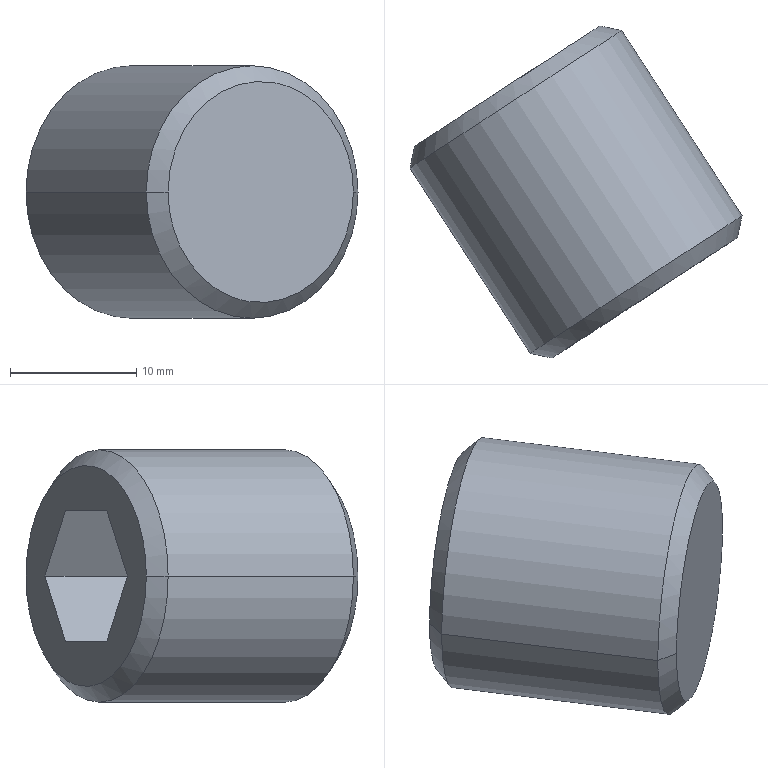Part | STEP file | Buj_o_1-A | 1 solid | 15 faces | box 26.305 x 26.305 x 20 mm | volume 4786 mm3 | plane 9 | cone 4 | cylinder 2 | commonest cylinder face diameters 20 x2
STEP:
#1=CARTESIAN_POINT('',(0.,0.,0.));
#2=DIRECTION('',(0.,0.,1.));
#3=DIRECTION('',(1.,0.,0.));
#4=AXIS2_PLACEMENT_3D('',#1,#2,#3);
#5=CARTESIAN_POINT('',(-85.7,150.327,23.));
#6=VERTEX_POINT('',#5);
#7=CARTESIAN_POINT('',(-102.473,139.434,23.));
#8=VERTEX_POINT('',#7);
#9=CARTESIAN_POINT('',(-94.086,144.88,23.));
#10=DIRECTION('',(0.5446,-0.8387,0.));
#11=DIRECTION('',(0.8387,0.5446,0.));
#12=AXIS2_PLACEMENT_3D('',#9,#10,#11);
#13=CIRCLE('',#12,10.);
#14=CARTESIAN_POINT('',(-94.767,145.929,23.));
#15=DIRECTION('',(0.5446,-0.8387,0.));
#16=DIRECTION('',(0.8387,0.5446,0.));
#17=AXIS2_PLACEMENT_3D('',#14,#15,#16);
#18=CYLINDRICAL_SURFACE('',#17,10.);
#19=CARTESIAN_POINT('',(0.,1.25));
#20=DIRECTION('',(1.,0.));
#21=VECTOR('',#20,1.);
#22=LINE('',#19,#21);
#23=(GEOMETRIC_REPRESENTATION_CONTEXT(2)PARAMETRIC_REPRESENTATION_CONTEXT()REPRESENTATION_CONTEXT('',''));
#24=DEFINITIONAL_REPRESENTATION('',(#22),#23);
#25=PCURVE('',#18,#24);
#26=CARTESIAN_POINT('',(-94.086,144.88,23.));
#27=DIRECTION('',(0.5446,-0.8387,0.));
#28=DIRECTION('',(0.8387,0.5446,0.));
#29=AXIS2_PLACEMENT_3D('',#26,#27,#28);
#30=CONICAL_SURFACE('',#29,10.,0.7854);
#31=CARTESIAN_POINT('',(0.,0.));
#32=DIRECTION('',(1.,0.));
#33=VECTOR('',#32,1.);
#34=LINE('',#31,#33);
#35=(GEOMETRIC_REPRESENTATION_CONTEXT(2)PARAMETRIC_REPRESENTATION_CONTEXT()REPRESENTATION_CONTEXT('',''));
#36=DEFINITIONAL_REPRESENTATION('',(#34),#35);
#37=PCURVE('',#30,#36);
#38=SURFACE_CURVE('',#13,(#25,#37),.PCURVE_S1.);
#39=EDGE_CURVE('',#6,#8,#38,.T.);
#40=ORIENTED_EDGE('',*,*,#39,.T.);
#41=CARTESIAN_POINT('',(-92.942,124.757,23.));
#42=VERTEX_POINT('',#41);
#43=CARTESIAN_POINT('',(-103.154,140.482,23.));
#44=DIRECTION('',(0.5446,-0.8387,0.));
#45=VECTOR('',#44,1.);
#46=LINE('',#43,#45);
#47=CARTESIAN_POINT('',(3.142,0.));
#48=DIRECTION('',(0.,1.));
#49=VECTOR('',#48,1.);
#50=LINE('',#47,#49);
#51=(GEOMETRIC_REPRESENTATION_CONTEXT(2)PARAMETRIC_REPRESENTATION_CONTEXT()REPRESENTATION_CONTEXT('',''));
#52=DEFINITIONAL_REPRESENTATION('',(#50),#51);
#53=PCURVE('',#18,#52);
#54=CARTESIAN_POINT('',(-94.767,145.929,23.));
#55=DIRECTION('',(0.5446,-0.8387,0.));
#56=DIRECTION('',(0.8387,0.5446,0.));
#57=AXIS2_PLACEMENT_3D('',#54,#55,#56);
#58=CYLINDRICAL_SURFACE('',#57,10.);
#59=CARTESIAN_POINT('',(3.142,0.));
#60=DIRECTION('',(0.,1.));
#61=VECTOR('',#60,1.);
#62=LINE('',#59,#61);
#63=(GEOMETRIC_REPRESENTATION_CONTEXT(2)PARAMETRIC_REPRESENTATION_CONTEXT()REPRESENTATION_CONTEXT('',''));
#64=DEFINITIONAL_REPRESENTATION('',(#62),#63);
#65=PCURVE('',#58,#64);
#66=SURFACE_CURVE('',#46,(#53,#65),.PCURVE_S1.);
#67=EDGE_CURVE('',#8,#42,#66,.T.);
#68=ORIENTED_EDGE('',*,*,#67,.T.);
#69=CARTESIAN_POINT('',(-76.169,135.65,23.));
#70=VERTEX_POINT('',#69);
#71=CARTESIAN_POINT('',(-84.555,130.204,23.));
#72=DIRECTION('',(-0.5446,0.8387,0.));
#73=DIRECTION('',(0.8387,0.5446,0.));
#74=AXIS2_PLACEMENT_3D('',#71,#72,#73);
#75=CIRCLE('',#74,10.);
#76=CARTESIAN_POINT('',(6.283,18.75));
#77=DIRECTION('',(-1.,0.));
#78=VECTOR('',#77,1.);
#79=LINE('',#76,#78);
#80=(GEOMETRIC_REPRESENTATION_CONTEXT(2)PARAMETRIC_REPRESENTATION_CONTEXT()REPRESENTATION_CONTEXT('',''));
#81=DEFINITIONAL_REPRESENTATION('',(#79),#80);
#82=PCURVE('',#18,#81);
#83=CARTESIAN_POINT('',(-84.555,130.204,23.));
#84=DIRECTION('',(-0.5446,0.8387,0.));
#85=DIRECTION('',(-0.8387,-0.5446,0.));
#86=AXIS2_PLACEMENT_3D('',#83,#84,#85);
#87=CONICAL_SURFACE('',#86,10.,0.7854);
#88=CARTESIAN_POINT('',(-3.142,0.));
#89=DIRECTION('',(1.,0.));
#90=VECTOR('',#89,1.);
#91=LINE('',#88,#90);
#92=(GEOMETRIC_REPRESENTATION_CONTEXT(2)PARAMETRIC_REPRESENTATION_CONTEXT()REPRESENTATION_CONTEXT('',''));
#93=DEFINITIONAL_REPRESENTATION('',(#91),#92);
#94=PCURVE('',#87,#93);
#95=SURFACE_CURVE('',#75,(#82,#94),.PCURVE_S1.);
#96=EDGE_CURVE('',#42,#70,#95,.T.);
#97=ORIENTED_EDGE('',*,*,#96,.T.);
#98=CARTESIAN_POINT('',(-86.38,151.375,23.));
#99=DIRECTION('',(0.5446,-0.8387,0.));
#100=VECTOR('',#99,1.);
#101=LINE('',#98,#100);
#102=CARTESIAN_POINT('',(0.,0.));
#103=DIRECTION('',(0.,1.));
#104=VECTOR('',#103,1.);
#105=LINE('',#102,#104);
#106=(GEOMETRIC_REPRESENTATION_CONTEXT(2)PARAMETRIC_REPRESENTATION_CONTEXT()REPRESENTATION_CONTEXT('',''));
#107=DEFINITIONAL_REPRESENTATION('',(#105),#106);
#108=PCURVE('',#18,#107);
#109=CARTESIAN_POINT('',(6.283,0.));
#110=DIRECTION('',(0.,1.));
#111=VECTOR('',#110,1.);
#112=LINE('',#109,#111);
#113=(GEOMETRIC_REPRESENTATION_CONTEXT(2)PARAMETRIC_REPRESENTATION_CONTEXT()REPRESENTATION_CONTEXT('',''));
#114=DEFINITIONAL_REPRESENTATION('',(#112),#113);
#115=PCURVE('',#58,#114);
#116=SURFACE_CURVE('',#101,(#108,#115),.PCURVE_S1.);
#117=EDGE_CURVE('',#6,#70,#116,.T.);
#118=ORIENTED_EDGE('',*,*,#117,.F.);
#119=EDGE_LOOP('',(#40,#68,#97,#118));
#120=FACE_BOUND('',#119,.T.);
#121=ADVANCED_FACE('',(#120),#18,.T.);
#122=CARTESIAN_POINT('',(-91.213,124.39,23.));
#123=VERTEX_POINT('',#122);
#124=CARTESIAN_POINT('',(-76.536,133.921,23.));
#125=VERTEX_POINT('',#124);
#126=CARTESIAN_POINT('',(-91.213,124.39,23.));
#127=CARTESIAN_POINT('',(-91.213,124.39,24.145));
#128=CARTESIAN_POINT('',(-91.022,124.514,25.29));
#129=CARTESIAN_POINT('',(-90.287,124.991,27.407));
#130=CARTESIAN_POINT('',(-89.743,125.344,28.377));
#131=CARTESIAN_POINT('',(-88.384,126.227,29.997));
#132=CARTESIAN_POINT('',(-87.57,126.755,30.646));
#133=CARTESIAN_POINT('',(-85.795,127.908,31.522));
#134=CARTESIAN_POINT('',(-84.835,128.531,31.75));
#135=CARTESIAN_POINT('',(-82.914,129.779,31.75));
#136=CARTESIAN_POINT('',(-81.954,130.403,31.522));
#137=CARTESIAN_POINT('',(-80.179,131.555,30.646));
#138=CARTESIAN_POINT('',(-79.365,132.084,29.997));
#139=CARTESIAN_POINT('',(-78.006,132.966,28.377));
#140=CARTESIAN_POINT('',(-77.462,133.319,27.407));
#141=CARTESIAN_POINT('',(-76.727,133.797,25.29));
#142=CARTESIAN_POINT('',(-76.536,133.921,24.145));
#143=CARTESIAN_POINT('',(-76.536,133.921,23.));
#144=B_SPLINE_CURVE_WITH_KNOTS('',3,(#126,#127,#128,#129,#130,#131,#132,#133,#134,#135,#136,#137,#138,#139,#140,#141,#142,#143),.UNSPECIFIED.,.F.,.F.,(4,2,2,2,2,2,2,2,4),(0.75,0.8125,0.875,0.9375,1.,1.062,1.125,1.188,1.25),.UNSPECIFIED.);
#145=CARTESIAN_POINT('',(0.,-1.25));
#146=CARTESIAN_POINT('',(0.0238,-1.25));
#147=CARTESIAN_POINT('',(0.0714,-1.25));
#148=CARTESIAN_POINT('',(0.1428,-1.25));
#149=CARTESIAN_POINT('',(0.2142,-1.25));
#150=CARTESIAN_POINT('',(0.2856,-1.25));
#151=CARTESIAN_POINT('',(0.357,-1.25));
#152=CARTESIAN_POINT('',(0.4284,-1.25));
#153=CARTESIAN_POINT('',(0.4998,-1.25));
#154=CARTESIAN_POINT('',(0.5712,-1.25));
#155=CARTESIAN_POINT('',(0.6426,-1.25));
#156=CARTESIAN_POINT('',(0.714,-1.25));
#157=CARTESIAN_POINT('',(0.7854,-1.25));
#158=CARTESIAN_POINT('',(0.8568,-1.25));
#159=CARTESIAN_POINT('',(0.9282,-1.25));
#160=CARTESIAN_POINT('',(0.9996,-1.25));
#161=CARTESIAN_POINT('',(1.071,-1.25));
#162=CARTESIAN_POINT('',(1.142,-1.25));
#163=CARTESIAN_POINT('',(1.214,-1.25));
#164=CARTESIAN_POINT('',(1.285,-1.25));
#165=CARTESIAN_POINT('',(1.357,-1.25));
#166=CARTESIAN_POINT('',(1.428,-1.25));
#167=CARTESIAN_POINT('',(1.499,-1.25));
#168=CARTESIAN_POINT('',(1.571,-1.25));
#169=CARTESIAN_POINT('',(1.642,-1.25));
#170=CARTESIAN_POINT('',(1.714,-1.25));
#171=CARTESIAN_POINT('',(1.785,-1.25));
#172=CARTESIAN_POINT('',(1.856,-1.25));
#173=CARTESIAN_POINT('',(1.928,-1.25));
#174=CARTESIAN_POINT('',(1.999,-1.25));
#175=CARTESIAN_POINT('',(2.071,-1.25));
#176=CARTESIAN_POINT('',(2.142,-1.25));
#177=CARTESIAN_POINT('',(2.213,-1.25));
#178=CARTESIAN_POINT('',(2.285,-1.25));
#179=CARTESIAN_POINT('',(2.356,-1.25));
#180=CARTESIAN_POINT('',(2.428,-1.25));
#181=CARTESIAN_POINT('',(2.499,-1.25));
#182=CARTESIAN_POINT('',(2.57,-1.25));
#183=CARTESIAN_POINT('',(2.642,-1.25));
#184=CARTESIAN_POINT('',(2.713,-1.25));
#185=CARTESIAN_POINT('',(2.785,-1.25));
#186=CARTESIAN_POINT('',(2.856,-1.25));
#187=CARTESIAN_POINT('',(2.927,-1.25));
#188=CARTESIAN_POINT('',(2.999,-1.25));
#189=CARTESIAN_POINT('',(3.07,-1.25));
#190=CARTESIAN_POINT('',(3.118,-1.25));
#191=CARTESIAN_POINT('',(3.142,-1.25));
#192=B_SPLINE_CURVE_WITH_KNOTS('',3,(#145,#146,#147,#148,#149,#150,#151,#152,#153,#154,#155,#156,#157,#158,#159,#160,#161,#162,#163,#164,#165,#166,#167,#168,#169,#170,#171,#172,#173,#174,#175,#176,#177,#178,#179,#180,#181,#182,#183,#184,#185,#186,#187,#188,#189,#190,#191),.UNSPECIFIED.,.F.,.F.,(4,1,1,1,1,1,1,1,1,1,1,1,1,1,1,1,1,1,1,1,1,1,1,1,1,1,1,1,1,1,1,1,1,1,1,1,1,1,1,1,1,1,1,1,4),(0.75,0.7614,0.7727,0.7841,0.7955,0.8068,0.8182,0.8295,0.8409,0.8523,0.8636,0.875,0.8864,0.8977,0.9091,0.9205,0.9318,0.9432,0.9545,0.9659,0.9773,0.9886,1.,1.011,1.023,1.034,1.045,1.057,1.068,1.08,1.091,1.102,1.114,1.125,1.136,1.148,1.159,1.17,1.182,1.193,1.205,1.216,1.227,1.239,1.25),.QUASI_UNIFORM_KNOTS.);
#193=(GEOMETRIC_REPRESENTATION_CONTEXT(2)PARAMETRIC_REPRESENTATION_CONTEXT()REPRESENTATION_CONTEXT('',''));
#194=DEFINITIONAL_REPRESENTATION('',(#192),#193);
#195=PCURVE('',#87,#194);
#196=CARTESIAN_POINT('',(-83.874,129.155,23.));
#197=DIRECTION('',(0.5446,-0.8387,0.));
#198=DIRECTION('',(0.8387,0.5446,0.));
#199=AXIS2_PLACEMENT_3D('',#196,#197,#198);
#200=PLANE('',#199);
#201=CARTESIAN_POINT('',(-8.75,0.));
#202=CARTESIAN_POINT('',(-8.75,1.145));
#203=CARTESIAN_POINT('',(-8.522,2.29));
#204=CARTESIAN_POINT('',(-7.646,4.407));
#205=CARTESIAN_POINT('',(-6.997,5.377));
#206=CARTESIAN_POINT('',(-5.377,6.997));
#207=CARTESIAN_POINT('',(-4.407,7.646));
#208=CARTESIAN_POINT('',(-2.29,8.522));
#209=CARTESIAN_POINT('',(-1.145,8.75));
#210=CARTESIAN_POINT('',(1.145,8.75));
#211=CARTESIAN_POINT('',(2.29,8.522));
#212=CARTESIAN_POINT('',(4.407,7.646));
#213=CARTESIAN_POINT('',(5.377,6.997));
#214=CARTESIAN_POINT('',(6.997,5.377));
#215=CARTESIAN_POINT('',(7.646,4.407));
#216=CARTESIAN_POINT('',(8.522,2.29));
#217=CARTESIAN_POINT('',(8.75,1.145));
#218=CARTESIAN_POINT('',(8.75,0.));
#219=B_SPLINE_CURVE_WITH_KNOTS('',3,(#201,#202,#203,#204,#205,#206,#207,#208,#209,#210,#211,#212,#213,#214,#215,#216,#217,#218),.UNSPECIFIED.,.F.,.F.,(4,2,2,2,2,2,2,2,4),(0.75,0.8125,0.875,0.9375,1.,1.062,1.125,1.188,1.25),.UNSPECIFIED.);
#220=(GEOMETRIC_REPRESENTATION_CONTEXT(2)PARAMETRIC_REPRESENTATION_CONTEXT()REPRESENTATION_CONTEXT('',''));
#221=DEFINITIONAL_REPRESENTATION('',(#219),#220);
#222=PCURVE('',#200,#221);
#223=SURFACE_CURVE('',#144,(#195,#222),.PCURVE_S1.);
#224=EDGE_CURVE('',#123,#125,#223,.T.);
#225=ORIENTED_EDGE('',*,*,#224,.T.);
#226=CARTESIAN_POINT('',(-76.169,135.65,23.));
#227=DIRECTION('',(0.2079,0.9781,0.));
#228=VECTOR('',#227,1.);
#229=LINE('',#226,#228);
#230=CARTESIAN_POINT('',(3.142,0.));
#231=DIRECTION('',(0.,1.));
#232=VECTOR('',#231,1.);
#233=LINE('',#230,#232);
#234=(GEOMETRIC_REPRESENTATION_CONTEXT(2)PARAMETRIC_REPRESENTATION_CONTEXT()REPRESENTATION_CONTEXT('',''));
#235=DEFINITIONAL_REPRESENTATION('',(#233),#234);
#236=PCURVE('',#87,#235);
#237=CARTESIAN_POINT('',(-84.555,130.204,23.));
#238=DIRECTION('',(-0.5446,0.8387,0.));
#239=DIRECTION('',(-0.8387,-0.5446,0.));
#240=AXIS2_PLACEMENT_3D('',#237,#238,#239);
#241=CONICAL_SURFACE('',#240,10.,0.7854);
#242=CARTESIAN_POINT('',(3.142,0.));
#243=DIRECTION('',(0.,1.));
#244=VECTOR('',#243,1.);
#245=LINE('',#242,#244);
#246=(GEOMETRIC_REPRESENTATION_CONTEXT(2)PARAMETRIC_REPRESENTATION_CONTEXT()REPRESENTATION_CONTEXT('',''));
#247=DEFINITIONAL_REPRESENTATION('',(#245),#246);
#248=PCURVE('',#241,#247);
#249=SURFACE_CURVE('',#229,(#236,#248),.PCURVE_S1.);
#250=EDGE_CURVE('',#125,#70,#249,.T.);
#251=ORIENTED_EDGE('',*,*,#250,.T.);
#252=ORIENTED_EDGE('',*,*,#96,.F.);
#253=CARTESIAN_POINT('',(-92.942,124.757,23.));
#254=DIRECTION('',(-0.9781,0.2079,0.));
#255=VECTOR('',#254,1.);
#256=LINE('',#253,#255);
#257=CARTESIAN_POINT('',(0.,0.));
#258=DIRECTION('',(0.,1.));
#259=VECTOR('',#258,1.);
#260=LINE('',#257,#259);
#261=(GEOMETRIC_REPRESENTATION_CONTEXT(2)PARAMETRIC_REPRESENTATION_CONTEXT()REPRESENTATION_CONTEXT('',''));
#262=DEFINITIONAL_REPRESENTATION('',(#260),#261);
#263=PCURVE('',#87,#262);
#264=CARTESIAN_POINT('',(6.283,0.));
#265=DIRECTION('',(0.,1.));
#266=VECTOR('',#265,1.);
#267=LINE('',#264,#266);
#268=(GEOMETRIC_REPRESENTATION_CONTEXT(2)PARAMETRIC_REPRESENTATION_CONTEXT()REPRESENTATION_CONTEXT('',''));
#269=DEFINITIONAL_REPRESENTATION('',(#267),#268);
#270=PCURVE('',#241,#269);
#271=SURFACE_CURVE('',#256,(#263,#270),.PCURVE_S1.);
#272=EDGE_CURVE('',#123,#42,#271,.T.);
#273=ORIENTED_EDGE('',*,*,#272,.F.);
#274=EDGE_LOOP('',(#225,#251,#252,#273));
#275=FACE_BOUND('',#274,.T.);
#276=ADVANCED_FACE('',(#275),#87,.T.);
#277=CARTESIAN_POINT('',(-87.429,150.694,23.));
#278=VERTEX_POINT('',#277);
#279=CARTESIAN_POINT('',(-102.106,141.163,23.));
#280=VERTEX_POINT('',#279);
#281=CARTESIAN_POINT('',(-87.429,150.694,23.));
#282=CARTESIAN_POINT('',(-87.429,150.694,24.145));
#283=CARTESIAN_POINT('',(-87.62,150.57,25.29));
#284=CARTESIAN_POINT('',(-88.355,150.093,27.407));
#285=CARTESIAN_POINT('',(-88.899,149.74,28.377));
#286=CARTESIAN_POINT('',(-90.257,148.857,29.997));
#287=CARTESIAN_POINT('',(-91.071,148.329,30.646));
#288=CARTESIAN_POINT('',(-92.846,147.176,31.522));
#289=CARTESIAN_POINT('',(-93.807,146.552,31.75));
#290=CARTESIAN_POINT('',(-95.728,145.305,31.75));
#291=CARTESIAN_POINT('',(-96.688,144.681,31.522));
#292=CARTESIAN_POINT('',(-98.463,143.529,30.646));
#293=CARTESIAN_POINT('',(-99.277,143.,29.997));
#294=CARTESIAN_POINT('',(-100.635,142.118,28.377));
#295=CARTESIAN_POINT('',(-101.179,141.765,27.407));
#296=CARTESIAN_POINT('',(-101.915,141.287,25.29));
#297=CARTESIAN_POINT('',(-102.106,141.163,24.145));
#298=CARTESIAN_POINT('',(-102.106,141.163,23.));
#299=B_SPLINE_CURVE_WITH_KNOTS('',3,(#281,#282,#283,#284,#285,#286,#287,#288,#289,#290,#291,#292,#293,#294,#295,#296,#297,#298),.UNSPECIFIED.,.F.,.F.,(4,2,2,2,2,2,2,2,4),(0.25,0.3125,0.375,0.4375,0.5,0.5625,0.625,0.6875,0.75),.UNSPECIFIED.);
#300=CARTESIAN_POINT('',(0.,-1.25));
#301=CARTESIAN_POINT('',(0.0238,-1.25));
#302=CARTESIAN_POINT('',(0.0714,-1.25));
#303=CARTESIAN_POINT('',(0.1428,-1.25));
#304=CARTESIAN_POINT('',(0.2142,-1.25));
#305=CARTESIAN_POINT('',(0.2856,-1.25));
#306=CARTESIAN_POINT('',(0.357,-1.25));
#307=CARTESIAN_POINT('',(0.4284,-1.25));
#308=CARTESIAN_POINT('',(0.4998,-1.25));
#309=CARTESIAN_POINT('',(0.5712,-1.25));
#310=CARTESIAN_POINT('',(0.6426,-1.25));
#311=CARTESIAN_POINT('',(0.714,-1.25));
#312=CARTESIAN_POINT('',(0.7854,-1.25));
#313=CARTESIAN_POINT('',(0.8568,-1.25));
#314=CARTESIAN_POINT('',(0.9282,-1.25));
#315=CARTESIAN_POINT('',(0.9996,-1.25));
#316=CARTESIAN_POINT('',(1.071,-1.25));
#317=CARTESIAN_POINT('',(1.142,-1.25));
#318=CARTESIAN_POINT('',(1.214,-1.25));
#319=CARTESIAN_POINT('',(1.285,-1.25));
#320=CARTESIAN_POINT('',(1.357,-1.25));
#321=CARTESIAN_POINT('',(1.428,-1.25));
#322=CARTESIAN_POINT('',(1.499,-1.25));
#323=CARTESIAN_POINT('',(1.571,-1.25));
#324=CARTESIAN_POINT('',(1.642,-1.25));
#325=CARTESIAN_POINT('',(1.714,-1.25));
#326=CARTESIAN_POINT('',(1.785,-1.25));
#327=CARTESIAN_POINT('',(1.856,-1.25));
#328=CARTESIAN_POINT('',(1.928,-1.25));
#329=CARTESIAN_POINT('',(1.999,-1.25));
#330=CARTESIAN_POINT('',(2.071,-1.25));
#331=CARTESIAN_POINT('',(2.142,-1.25));
#332=CARTESIAN_POINT('',(2.213,-1.25));
#333=CARTESIAN_POINT('',(2.285,-1.25));
#334=CARTESIAN_POINT('',(2.356,-1.25));
#335=CARTESIAN_POINT('',(2.428,-1.25));
#336=CARTESIAN_POINT('',(2.499,-1.25));
#337=CARTESIAN_POINT('',(2.57,-1.25));
#338=CARTESIAN_POINT('',(2.642,-1.25));
#339=CARTESIAN_POINT('',(2.713,-1.25));
#340=CARTESIAN_POINT('',(2.785,-1.25));
#341=CARTESIAN_POINT('',(2.856,-1.25));
#342=CARTESIAN_POINT('',(2.927,-1.25));
#343=CARTESIAN_POINT('',(2.999,-1.25));
#344=CARTESIAN_POINT('',(3.07,-1.25));
#345=CARTESIAN_POINT('',(3.118,-1.25));
#346=CARTESIAN_POINT('',(3.142,-1.25));
#347=B_SPLINE_CURVE_WITH_KNOTS('',3,(#300,#301,#302,#303,#304,#305,#306,#307,#308,#309,#310,#311,#312,#313,#314,#315,#316,#317,#318,#319,#320,#321,#322,#323,#324,#325,#326,#327,#328,#329,#330,#331,#332,#333,#334,#335,#336,#337,#338,#339,#340,#341,#342,#343,#344,#345,#346),.UNSPECIFIED.,.F.,.F.,(4,1,1,1,1,1,1,1,1,1,1,1,1,1,1,1,1,1,1,1,1,1,1,1,1,1,1,1,1,1,1,1,1,1,1,1,1,1,1,1,1,1,1,1,4),(0.25,0.2614,0.2727,0.2841,0.2955,0.3068,0.3182,0.3295,0.3409,0.3523,0.3636,0.375,0.3864,0.3977,0.4091,0.4205,0.4318,0.4432,0.4545,0.4659,0.4773,0.4886,0.5,0.5114,0.5227,0.5341,0.5455,0.5568,0.5682,0.5795,0.5909,0.6023,0.6136,0.625,0.6364,0.6477,0.6591,0.6705,0.6818,0.6932,0.7045,0.7159,0.7273,0.7386,0.75),.QUASI_UNIFORM_KNOTS.);
#348=(GEOMETRIC_REPRESENTATION_CONTEXT(2)PARAMETRIC_REPRESENTATION_CONTEXT()REPRESENTATION_CONTEXT('',''));
#349=DEFINITIONAL_REPRESENTATION('',(#347),#348);
#350=PCURVE('',#30,#349);
#351=CARTESIAN_POINT('',(-94.767,145.929,23.));
#352=DIRECTION('',(-0.5446,0.8387,0.));
#353=DIRECTION('',(-0.8387,-0.5446,0.));
#354=AXIS2_PLACEMENT_3D('',#351,#352,#353);
#355=PLANE('',#354);
#356=CARTESIAN_POINT('',(-8.75,0.));
#357=CARTESIAN_POINT('',(-8.75,1.145));
#358=CARTESIAN_POINT('',(-8.522,2.29));
#359=CARTESIAN_POINT('',(-7.646,4.407));
#360=CARTESIAN_POINT('',(-6.997,5.377));
#361=CARTESIAN_POINT('',(-5.377,6.997));
#362=CARTESIAN_POINT('',(-4.407,7.646));
#363=CARTESIAN_POINT('',(-2.29,8.522));
#364=CARTESIAN_POINT('',(-1.145,8.75));
#365=CARTESIAN_POINT('',(1.145,8.75));
#366=CARTESIAN_POINT('',(2.29,8.522));
#367=CARTESIAN_POINT('',(4.407,7.646));
#368=CARTESIAN_POINT('',(5.377,6.997));
#369=CARTESIAN_POINT('',(6.997,5.377));
#370=CARTESIAN_POINT('',(7.646,4.407));
#371=CARTESIAN_POINT('',(8.522,2.29));
#372=CARTESIAN_POINT('',(8.75,1.145));
#373=CARTESIAN_POINT('',(8.75,0.));
#374=B_SPLINE_CURVE_WITH_KNOTS('',3,(#356,#357,#358,#359,#360,#361,#362,#363,#364,#365,#366,#367,#368,#369,#370,#371,#372,#373),.UNSPECIFIED.,.F.,.F.,(4,2,2,2,2,2,2,2,4),(0.25,0.3125,0.375,0.4375,0.5,0.5625,0.625,0.6875,0.75),.UNSPECIFIED.);
#375=(GEOMETRIC_REPRESENTATION_CONTEXT(2)PARAMETRIC_REPRESENTATION_CONTEXT()REPRESENTATION_CONTEXT('',''));
#376=DEFINITIONAL_REPRESENTATION('',(#374),#375);
#377=PCURVE('',#355,#376);
#378=SURFACE_CURVE('',#299,(#350,#377),.PCURVE_S1.);
#379=EDGE_CURVE('',#278,#280,#378,.T.);
#380=ORIENTED_EDGE('',*,*,#379,.T.);
#381=CARTESIAN_POINT('',(-102.473,139.434,23.));
#382=DIRECTION('',(-0.2079,-0.9781,0.));
#383=VECTOR('',#382,1.);
#384=LINE('',#381,#383);
#385=CARTESIAN_POINT('',(3.142,0.));
#386=DIRECTION('',(0.,1.));
#387=VECTOR('',#386,1.);
#388=LINE('',#385,#387);
#389=(GEOMETRIC_REPRESENTATION_CONTEXT(2)PARAMETRIC_REPRESENTATION_CONTEXT()REPRESENTATION_CONTEXT('',''));
#390=DEFINITIONAL_REPRESENTATION('',(#388),#389);
#391=PCURVE('',#30,#390);
#392=CARTESIAN_POINT('',(-94.086,144.88,23.));
#393=DIRECTION('',(0.5446,-0.8387,0.));
#394=DIRECTION('',(0.8387,0.5446,0.));
#395=AXIS2_PLACEMENT_3D('',#392,#393,#394);
#396=CONICAL_SURFACE('',#395,10.,0.7854);
#397=CARTESIAN_POINT('',(3.142,0.));
#398=DIRECTION('',(0.,1.));
#399=VECTOR('',#398,1.);
#400=LINE('',#397,#399);
#401=(GEOMETRIC_REPRESENTATION_CONTEXT(2)PARAMETRIC_REPRESENTATION_CONTEXT()REPRESENTATION_CONTEXT('',''));
#402=DEFINITIONAL_REPRESENTATION('',(#400),#401);
#403=PCURVE('',#396,#402);
#404=SURFACE_CURVE('',#384,(#391,#403),.PCURVE_S1.);
#405=EDGE_CURVE('',#280,#8,#404,.T.);
#406=ORIENTED_EDGE('',*,*,#405,.T.);
#407=ORIENTED_EDGE('',*,*,#39,.F.);
#408=CARTESIAN_POINT('',(-85.7,150.327,23.));
#409=DIRECTION('',(0.9781,-0.2079,0.));
#410=VECTOR('',#409,1.);
#411=LINE('',#408,#410);
#412=CARTESIAN_POINT('',(0.,0.));
#413=DIRECTION('',(0.,1.));
#414=VECTOR('',#413,1.);
#415=LINE('',#412,#414);
#416=(GEOMETRIC_REPRESENTATION_CONTEXT(2)PARAMETRIC_REPRESENTATION_CONTEXT()REPRESENTATION_CONTEXT('',''));
#417=DEFINITIONAL_REPRESENTATION('',(#415),#416);
#418=PCURVE('',#30,#417);
#419=CARTESIAN_POINT('',(6.283,0.));
#420=DIRECTION('',(0.,1.));
#421=VECTOR('',#420,1.);
#422=LINE('',#419,#421);
#423=(GEOMETRIC_REPRESENTATION_CONTEXT(2)PARAMETRIC_REPRESENTATION_CONTEXT()REPRESENTATION_CONTEXT('',''));
#424=DEFINITIONAL_REPRESENTATION('',(#422),#423);
#425=PCURVE('',#396,#424);
#426=SURFACE_CURVE('',#411,(#418,#425),.PCURVE_S1.);
#427=EDGE_CURVE('',#278,#6,#426,.T.);
#428=ORIENTED_EDGE('',*,*,#427,.F.);
#429=EDGE_LOOP('',(#380,#406,#407,#428));
#430=FACE_BOUND('',#429,.T.);
#431=ADVANCED_FACE('',(#430),#30,.T.);
#432=ORIENTED_EDGE('',*,*,#67,.F.);
#433=CARTESIAN_POINT('',(-94.086,144.88,23.));
#434=DIRECTION('',(0.5446,-0.8387,0.));
#435=DIRECTION('',(0.8387,0.5446,0.));
#436=AXIS2_PLACEMENT_3D('',#433,#434,#435);
#437=CIRCLE('',#436,10.);
#438=CARTESIAN_POINT('',(0.,1.25));
#439=DIRECTION('',(1.,0.));
#440=VECTOR('',#439,1.);
#441=LINE('',#438,#440);
#442=(GEOMETRIC_REPRESENTATION_CONTEXT(2)PARAMETRIC_REPRESENTATION_CONTEXT()REPRESENTATION_CONTEXT('',''));
#443=DEFINITIONAL_REPRESENTATION('',(#441),#442);
#444=PCURVE('',#58,#443);
#445=CARTESIAN_POINT('',(0.,0.));
#446=DIRECTION('',(1.,0.));
#447=VECTOR('',#446,1.);
#448=LINE('',#445,#447);
#449=(GEOMETRIC_REPRESENTATION_CONTEXT(2)PARAMETRIC_REPRESENTATION_CONTEXT()REPRESENTATION_CONTEXT('',''));
#450=DEFINITIONAL_REPRESENTATION('',(#448),#449);
#451=PCURVE('',#396,#450);
#452=SURFACE_CURVE('',#437,(#444,#451),.PCURVE_S1.);
#453=EDGE_CURVE('',#8,#6,#452,.T.);
#454=ORIENTED_EDGE('',*,*,#453,.T.);
#455=ORIENTED_EDGE('',*,*,#117,.T.);
#456=CARTESIAN_POINT('',(-84.555,130.204,23.));
#457=DIRECTION('',(-0.5446,0.8387,0.));
#458=DIRECTION('',(0.8387,0.5446,0.));
#459=AXIS2_PLACEMENT_3D('',#456,#457,#458);
#460=CIRCLE('',#459,10.);
#461=CARTESIAN_POINT('',(6.283,18.75));
#462=DIRECTION('',(-1.,0.));
#463=VECTOR('',#462,1.);
#464=LINE('',#461,#463);
#465=(GEOMETRIC_REPRESENTATION_CONTEXT(2)PARAMETRIC_REPRESENTATION_CONTEXT()REPRESENTATION_CONTEXT('',''));
#466=DEFINITIONAL_REPRESENTATION('',(#464),#465);
#467=PCURVE('',#58,#466);
#468=CARTESIAN_POINT('',(3.142,0.));
#469=DIRECTION('',(1.,0.));
#470=VECTOR('',#469,1.);
#471=LINE('',#468,#470);
#472=(GEOMETRIC_REPRESENTATION_CONTEXT(2)PARAMETRIC_REPRESENTATION_CONTEXT()REPRESENTATION_CONTEXT('',''));
#473=DEFINITIONAL_REPRESENTATION('',(#471),#472);
#474=PCURVE('',#241,#473);
#475=SURFACE_CURVE('',#460,(#467,#474),.PCURVE_S1.);
#476=EDGE_CURVE('',#70,#42,#475,.T.);
#477=ORIENTED_EDGE('',*,*,#476,.T.);
#478=EDGE_LOOP('',(#432,#454,#455,#477));
#479=FACE_BOUND('',#478,.T.);
#480=ADVANCED_FACE('',(#479),#58,.T.);
#481=ORIENTED_EDGE('',*,*,#250,.F.);
#482=CARTESIAN_POINT('',(-76.536,133.921,23.));
#483=CARTESIAN_POINT('',(-76.536,133.921,21.855));
#484=CARTESIAN_POINT('',(-76.727,133.797,20.71));
#485=CARTESIAN_POINT('',(-77.462,133.319,18.593));
#486=CARTESIAN_POINT('',(-78.006,132.966,17.623));
#487=CARTESIAN_POINT('',(-79.365,132.084,16.003));
#488=CARTESIAN_POINT('',(-80.179,131.555,15.354));
#489=CARTESIAN_POINT('',(-81.954,130.403,14.478));
#490=CARTESIAN_POINT('',(-82.914,129.779,14.25));
#491=CARTESIAN_POINT('',(-84.835,128.531,14.25));
#492=CARTESIAN_POINT('',(-85.795,127.908,14.478));
#493=CARTESIAN_POINT('',(-87.57,126.755,15.354));
#494=CARTESIAN_POINT('',(-88.384,126.227,16.003));
#495=CARTESIAN_POINT('',(-89.743,125.344,17.623));
#496=CARTESIAN_POINT('',(-90.287,124.991,18.593));
#497=CARTESIAN_POINT('',(-91.022,124.514,20.71));
#498=CARTESIAN_POINT('',(-91.213,124.39,21.855));
#499=CARTESIAN_POINT('',(-91.213,124.39,23.));
#500=B_SPLINE_CURVE_WITH_KNOTS('',3,(#482,#483,#484,#485,#486,#487,#488,#489,#490,#491,#492,#493,#494,#495,#496,#497,#498,#499),.UNSPECIFIED.,.F.,.F.,(4,2,2,2,2,2,2,2,4),(0.25,0.3125,0.375,0.4375,0.5,0.5625,0.625,0.6875,0.75),.UNSPECIFIED.);
#501=CARTESIAN_POINT('',(3.142,-1.25));
#502=CARTESIAN_POINT('',(3.165,-1.25));
#503=CARTESIAN_POINT('',(3.213,-1.25));
#504=CARTESIAN_POINT('',(3.284,-1.25));
#505=CARTESIAN_POINT('',(3.356,-1.25));
#506=CARTESIAN_POINT('',(3.427,-1.25));
#507=CARTESIAN_POINT('',(3.499,-1.25));
#508=CARTESIAN_POINT('',(3.57,-1.25));
#509=CARTESIAN_POINT('',(3.641,-1.25));
#510=CARTESIAN_POINT('',(3.713,-1.25));
#511=CARTESIAN_POINT('',(3.784,-1.25));
#512=CARTESIAN_POINT('',(3.856,-1.25));
#513=CARTESIAN_POINT('',(3.927,-1.25));
#514=CARTESIAN_POINT('',(3.998,-1.25));
#515=CARTESIAN_POINT('',(4.07,-1.25));
#516=CARTESIAN_POINT('',(4.141,-1.25));
#517=CARTESIAN_POINT('',(4.213,-1.25));
#518=CARTESIAN_POINT('',(4.284,-1.25));
#519=CARTESIAN_POINT('',(4.355,-1.25));
#520=CARTESIAN_POINT('',(4.427,-1.25));
#521=CARTESIAN_POINT('',(4.498,-1.25));
#522=CARTESIAN_POINT('',(4.57,-1.25));
#523=CARTESIAN_POINT('',(4.641,-1.25));
#524=CARTESIAN_POINT('',(4.712,-1.25));
#525=CARTESIAN_POINT('',(4.784,-1.25));
#526=CARTESIAN_POINT('',(4.855,-1.25));
#527=CARTESIAN_POINT('',(4.927,-1.25));
#528=CARTESIAN_POINT('',(4.998,-1.25));
#529=CARTESIAN_POINT('',(5.069,-1.25));
#530=CARTESIAN_POINT('',(5.141,-1.25));
#531=CARTESIAN_POINT('',(5.212,-1.25));
#532=CARTESIAN_POINT('',(5.284,-1.25));
#533=CARTESIAN_POINT('',(5.355,-1.25));
#534=CARTESIAN_POINT('',(5.426,-1.25));
#535=CARTESIAN_POINT('',(5.498,-1.25));
#536=CARTESIAN_POINT('',(5.569,-1.25));
#537=CARTESIAN_POINT('',(5.641,-1.25));
#538=CARTESIAN_POINT('',(5.712,-1.25));
#539=CARTESIAN_POINT('',(5.783,-1.25));
#540=CARTESIAN_POINT('',(5.855,-1.25));
#541=CARTESIAN_POINT('',(5.926,-1.25));
#542=CARTESIAN_POINT('',(5.998,-1.25));
#543=CARTESIAN_POINT('',(6.069,-1.25));
#544=CARTESIAN_POINT('',(6.14,-1.25));
#545=CARTESIAN_POINT('',(6.212,-1.25));
#546=CARTESIAN_POINT('',(6.259,-1.25));
#547=CARTESIAN_POINT('',(6.283,-1.25));
#548=B_SPLINE_CURVE_WITH_KNOTS('',3,(#501,#502,#503,#504,#505,#506,#507,#508,#509,#510,#511,#512,#513,#514,#515,#516,#517,#518,#519,#520,#521,#522,#523,#524,#525,#526,#527,#528,#529,#530,#531,#532,#533,#534,#535,#536,#537,#538,#539,#540,#541,#542,#543,#544,#545,#546,#547),.UNSPECIFIED.,.F.,.F.,(4,1,1,1,1,1,1,1,1,1,1,1,1,1,1,1,1,1,1,1,1,1,1,1,1,1,1,1,1,1,1,1,1,1,1,1,1,1,1,1,1,1,1,1,4),(0.25,0.2614,0.2727,0.2841,0.2955,0.3068,0.3182,0.3295,0.3409,0.3523,0.3636,0.375,0.3864,0.3977,0.4091,0.4205,0.4318,0.4432,0.4545,0.4659,0.4773,0.4886,0.5,0.5114,0.5227,0.5341,0.5455,0.5568,0.5682,0.5795,0.5909,0.6023,0.6136,0.625,0.6364,0.6477,0.6591,0.6705,0.6818,0.6932,0.7045,0.7159,0.7273,0.7386,0.75),.QUASI_UNIFORM_KNOTS.);
#549=(GEOMETRIC_REPRESENTATION_CONTEXT(2)PARAMETRIC_REPRESENTATION_CONTEXT()REPRESENTATION_CONTEXT('',''));
#550=DEFINITIONAL_REPRESENTATION('',(#548),#549);
#551=PCURVE('',#241,#550);
#552=CARTESIAN_POINT('',(8.75,0.));
#553=CARTESIAN_POINT('',(8.75,-1.145));
#554=CARTESIAN_POINT('',(8.522,-2.29));
#555=CARTESIAN_POINT('',(7.646,-4.407));
#556=CARTESIAN_POINT('',(6.997,-5.377));
#557=CARTESIAN_POINT('',(5.377,-6.997));
#558=CARTESIAN_POINT('',(4.407,-7.646));
#559=CARTESIAN_POINT('',(2.29,-8.522));
#560=CARTESIAN_POINT('',(1.145,-8.75));
#561=CARTESIAN_POINT('',(-1.145,-8.75));
#562=CARTESIAN_POINT('',(-2.29,-8.522));
#563=CARTESIAN_POINT('',(-4.407,-7.646));
#564=CARTESIAN_POINT('',(-5.377,-6.997));
#565=CARTESIAN_POINT('',(-6.997,-5.377));
#566=CARTESIAN_POINT('',(-7.646,-4.407));
#567=CARTESIAN_POINT('',(-8.522,-2.29));
#568=CARTESIAN_POINT('',(-8.75,-1.145));
#569=CARTESIAN_POINT('',(-8.75,0.));
#570=B_SPLINE_CURVE_WITH_KNOTS('',3,(#552,#553,#554,#555,#556,#557,#558,#559,#560,#561,#562,#563,#564,#565,#566,#567,#568,#569),.UNSPECIFIED.,.F.,.F.,(4,2,2,2,2,2,2,2,4),(0.25,0.3125,0.375,0.4375,0.5,0.5625,0.625,0.6875,0.75),.UNSPECIFIED.);
#571=(GEOMETRIC_REPRESENTATION_CONTEXT(2)PARAMETRIC_REPRESENTATION_CONTEXT()REPRESENTATION_CONTEXT('',''));
#572=DEFINITIONAL_REPRESENTATION('',(#570),#571);
#573=PCURVE('',#200,#572);
#574=SURFACE_CURVE('',#500,(#551,#573),.PCURVE_S1.);
#575=EDGE_CURVE('',#125,#123,#574,.T.);
#576=ORIENTED_EDGE('',*,*,#575,.T.);
#577=ORIENTED_EDGE('',*,*,#272,.T.);
#578=ORIENTED_EDGE('',*,*,#476,.F.);
#579=EDGE_LOOP('',(#481,#576,#577,#578));
#580=FACE_BOUND('',#579,.T.);
#581=ADVANCED_FACE('',(#580),#241,.T.);
#582=ORIENTED_EDGE('',*,*,#405,.F.);
#583=CARTESIAN_POINT('',(-102.106,141.163,23.));
#584=CARTESIAN_POINT('',(-102.106,141.163,21.855));
#585=CARTESIAN_POINT('',(-101.915,141.287,20.71));
#586=CARTESIAN_POINT('',(-101.179,141.765,18.593));
#587=CARTESIAN_POINT('',(-100.635,142.118,17.623));
#588=CARTESIAN_POINT('',(-99.277,143.,16.003));
#589=CARTESIAN_POINT('',(-98.463,143.529,15.354));
#590=CARTESIAN_POINT('',(-96.688,144.681,14.478));
#591=CARTESIAN_POINT('',(-95.728,145.305,14.25));
#592=CARTESIAN_POINT('',(-93.807,146.552,14.25));
#593=CARTESIAN_POINT('',(-92.846,147.176,14.478));
#594=CARTESIAN_POINT('',(-91.071,148.329,15.354));
#595=CARTESIAN_POINT('',(-90.257,148.857,16.003));
#596=CARTESIAN_POINT('',(-88.899,149.74,17.623));
#597=CARTESIAN_POINT('',(-88.355,150.093,18.593));
#598=CARTESIAN_POINT('',(-87.62,150.57,20.71));
#599=CARTESIAN_POINT('',(-87.429,150.694,21.855));
#600=CARTESIAN_POINT('',(-87.429,150.694,23.));
#601=B_SPLINE_CURVE_WITH_KNOTS('',3,(#583,#584,#585,#586,#587,#588,#589,#590,#591,#592,#593,#594,#595,#596,#597,#598,#599,#600),.UNSPECIFIED.,.F.,.F.,(4,2,2,2,2,2,2,2,4),(0.75,0.8125,0.875,0.9375,1.,1.062,1.125,1.188,1.25),.UNSPECIFIED.);
#602=CARTESIAN_POINT('',(3.142,-1.25));
#603=CARTESIAN_POINT('',(3.165,-1.25));
#604=CARTESIAN_POINT('',(3.213,-1.25));
#605=CARTESIAN_POINT('',(3.284,-1.25));
#606=CARTESIAN_POINT('',(3.356,-1.25));
#607=CARTESIAN_POINT('',(3.427,-1.25));
#608=CARTESIAN_POINT('',(3.499,-1.25));
#609=CARTESIAN_POINT('',(3.57,-1.25));
#610=CARTESIAN_POINT('',(3.641,-1.25));
#611=CARTESIAN_POINT('',(3.713,-1.25));
#612=CARTESIAN_POINT('',(3.784,-1.25));
#613=CARTESIAN_POINT('',(3.856,-1.25));
#614=CARTESIAN_POINT('',(3.927,-1.25));
#615=CARTESIAN_POINT('',(3.998,-1.25));
#616=CARTESIAN_POINT('',(4.07,-1.25));
#617=CARTESIAN_POINT('',(4.141,-1.25));
#618=CARTESIAN_POINT('',(4.213,-1.25));
#619=CARTESIAN_POINT('',(4.284,-1.25));
#620=CARTESIAN_POINT('',(4.355,-1.25));
#621=CARTESIAN_POINT('',(4.427,-1.25));
#622=CARTESIAN_POINT('',(4.498,-1.25));
#623=CARTESIAN_POINT('',(4.57,-1.25));
#624=CARTESIAN_POINT('',(4.641,-1.25));
#625=CARTESIAN_POINT('',(4.712,-1.25));
#626=CARTESIAN_POINT('',(4.784,-1.25));
#627=CARTESIAN_POINT('',(4.855,-1.25));
#628=CARTESIAN_POINT('',(4.927,-1.25));
#629=CARTESIAN_POINT('',(4.998,-1.25));
#630=CARTESIAN_POINT('',(5.069,-1.25));
#631=CARTESIAN_POINT('',(5.141,-1.25));
#632=CARTESIAN_POINT('',(5.212,-1.25));
#633=CARTESIAN_POINT('',(5.284,-1.25));
#634=CARTESIAN_POINT('',(5.355,-1.25));
#635=CARTESIAN_POINT('',(5.426,-1.25));
#636=CARTESIAN_POINT('',(5.498,-1.25));
#637=CARTESIAN_POINT('',(5.569,-1.25));
#638=CARTESIAN_POINT('',(5.641,-1.25));
#639=CARTESIAN_POINT('',(5.712,-1.25));
#640=CARTESIAN_POINT('',(5.783,-1.25));
#641=CARTESIAN_POINT('',(5.855,-1.25));
#642=CARTESIAN_POINT('',(5.926,-1.25));
#643=CARTESIAN_POINT('',(5.998,-1.25));
#644=CARTESIAN_POINT('',(6.069,-1.25));
#645=CARTESIAN_POINT('',(6.14,-1.25));
#646=CARTESIAN_POINT('',(6.212,-1.25));
#647=CARTESIAN_POINT('',(6.259,-1.25));
#648=CARTESIAN_POINT('',(6.283,-1.25));
#649=B_SPLINE_CURVE_WITH_KNOTS('',3,(#602,#603,#604,#605,#606,#607,#608,#609,#610,#611,#612,#613,#614,#615,#616,#617,#618,#619,#620,#621,#622,#623,#624,#625,#626,#627,#628,#629,#630,#631,#632,#633,#634,#635,#636,#637,#638,#639,#640,#641,#642,#643,#644,#645,#646,#647,#648),.UNSPECIFIED.,.F.,.F.,(4,1,1,1,1,1,1,1,1,1,1,1,1,1,1,1,1,1,1,1,1,1,1,1,1,1,1,1,1,1,1,1,1,1,1,1,1,1,1,1,1,1,1,1,4),(0.75,0.7614,0.7727,0.7841,0.7955,0.8068,0.8182,0.8295,0.8409,0.8523,0.8636,0.875,0.8864,0.8977,0.9091,0.9205,0.9318,0.9432,0.9545,0.9659,0.9773,0.9886,1.,1.011,1.023,1.034,1.045,1.057,1.068,1.08,1.091,1.102,1.114,1.125,1.136,1.148,1.159,1.17,1.182,1.193,1.205,1.216,1.227,1.239,1.25),.QUASI_UNIFORM_KNOTS.);
#650=(GEOMETRIC_REPRESENTATION_CONTEXT(2)PARAMETRIC_REPRESENTATION_CONTEXT()REPRESENTATION_CONTEXT('',''));
#651=DEFINITIONAL_REPRESENTATION('',(#649),#650);
#652=PCURVE('',#396,#651);
#653=CARTESIAN_POINT('',(8.75,0.));
#654=CARTESIAN_POINT('',(8.75,-1.145));
#655=CARTESIAN_POINT('',(8.522,-2.29));
#656=CARTESIAN_POINT('',(7.646,-4.407));
#657=CARTESIAN_POINT('',(6.997,-5.377));
#658=CARTESIAN_POINT('',(5.377,-6.997));
#659=CARTESIAN_POINT('',(4.407,-7.646));
#660=CARTESIAN_POINT('',(2.29,-8.522));
#661=CARTESIAN_POINT('',(1.145,-8.75));
#662=CARTESIAN_POINT('',(-1.145,-8.75));
#663=CARTESIAN_POINT('',(-2.29,-8.522));
#664=CARTESIAN_POINT('',(-4.407,-7.646));
#665=CARTESIAN_POINT('',(-5.377,-6.997));
#666=CARTESIAN_POINT('',(-6.997,-5.377));
#667=CARTESIAN_POINT('',(-7.646,-4.407));
#668=CARTESIAN_POINT('',(-8.522,-2.29));
#669=CARTESIAN_POINT('',(-8.75,-1.145));
#670=CARTESIAN_POINT('',(-8.75,0.));
#671=B_SPLINE_CURVE_WITH_KNOTS('',3,(#653,#654,#655,#656,#657,#658,#659,#660,#661,#662,#663,#664,#665,#666,#667,#668,#669,#670),.UNSPECIFIED.,.F.,.F.,(4,2,2,2,2,2,2,2,4),(0.75,0.8125,0.875,0.9375,1.,1.062,1.125,1.188,1.25),.UNSPECIFIED.);
#672=(GEOMETRIC_REPRESENTATION_CONTEXT(2)PARAMETRIC_REPRESENTATION_CONTEXT()REPRESENTATION_CONTEXT('',''));
#673=DEFINITIONAL_REPRESENTATION('',(#671),#672);
#674=PCURVE('',#355,#673);
#675=SURFACE_CURVE('',#601,(#652,#674),.PCURVE_S1.);
#676=EDGE_CURVE('',#280,#278,#675,.T.);
#677=ORIENTED_EDGE('',*,*,#676,.T.);
#678=ORIENTED_EDGE('',*,*,#427,.T.);
#679=ORIENTED_EDGE('',*,*,#453,.F.);
#680=EDGE_LOOP('',(#582,#677,#678,#679));
#681=FACE_BOUND('',#680,.T.);
#682=ADVANCED_FACE('',(#681),#396,.T.);
#683=ORIENTED_EDGE('',*,*,#224,.F.);
#684=ORIENTED_EDGE('',*,*,#575,.F.);
#685=EDGE_LOOP('',(#683,#684));
#686=FACE_BOUND('',#685,.T.);
#687=ADVANCED_FACE('',(#686),#200,.T.);
#688=ORIENTED_EDGE('',*,*,#379,.F.);
#689=ORIENTED_EDGE('',*,*,#676,.F.);
#690=EDGE_LOOP('',(#688,#689));
#691=FACE_BOUND('',#690,.T.);
#692=CARTESIAN_POINT('',(-92.251,147.563,28.196));
#693=VERTEX_POINT('',#692);
#694=CARTESIAN_POINT('',(-97.283,144.295,28.196));
#695=VERTEX_POINT('',#694);
#696=CARTESIAN_POINT('',(-94.767,145.929,28.196));
#697=DIRECTION('',(-0.8387,-0.5446,0.));
#698=VECTOR('',#697,1.);
#699=LINE('',#696,#698);
#700=CARTESIAN_POINT('',(0.,5.196));
#701=DIRECTION('',(1.,0.));
#702=VECTOR('',#701,1.);
#703=LINE('',#700,#702);
#704=(GEOMETRIC_REPRESENTATION_CONTEXT(2)PARAMETRIC_REPRESENTATION_CONTEXT()REPRESENTATION_CONTEXT('',''));
#705=DEFINITIONAL_REPRESENTATION('',(#703),#704);
#706=PCURVE('',#355,#705);
#707=CARTESIAN_POINT('',(-97.283,144.295,28.196));
#708=DIRECTION('',(0.,0.,-1.));
#709=DIRECTION('',(0.,1.,0.));
#710=AXIS2_PLACEMENT_3D('',#707,#708,#709);
#711=PLANE('',#710);
#712=CARTESIAN_POINT('',(1.634,2.516));
#713=DIRECTION('',(-0.5446,-0.8387));
#714=VECTOR('',#713,1.);
#715=LINE('',#712,#714);
#716=(GEOMETRIC_REPRESENTATION_CONTEXT(2)PARAMETRIC_REPRESENTATION_CONTEXT()REPRESENTATION_CONTEXT('',''));
#717=DEFINITIONAL_REPRESENTATION('',(#715),#716);
#718=PCURVE('',#711,#717);
#719=SURFACE_CURVE('',#699,(#706,#718),.PCURVE_S1.);
#720=EDGE_CURVE('',#693,#695,#719,.T.);
#721=ORIENTED_EDGE('',*,*,#720,.T.);
#722=CARTESIAN_POINT('',(-99.799,142.661,23.));
#723=VERTEX_POINT('',#722);
#724=CARTESIAN_POINT('',(-97.283,144.295,28.196));
#725=DIRECTION('',(-0.4193,-0.2723,-0.866));
#726=VECTOR('',#725,1.);
#727=LINE('',#724,#726);
#728=CARTESIAN_POINT('',(3.,5.196));
#729=DIRECTION('',(0.5,-0.866));
#730=VECTOR('',#729,1.);
#731=LINE('',#728,#730);
#732=(GEOMETRIC_REPRESENTATION_CONTEXT(2)PARAMETRIC_REPRESENTATION_CONTEXT()REPRESENTATION_CONTEXT('',''));
#733=DEFINITIONAL_REPRESENTATION('',(#731),#732);
#734=PCURVE('',#355,#733);
#735=CARTESIAN_POINT('',(-99.799,142.661,23.));
#736=DIRECTION('',(0.7263,0.4717,-0.5));
#737=DIRECTION('',(-0.567,0.,-0.8237));
#738=AXIS2_PLACEMENT_3D('',#735,#736,#737);
#739=PLANE('',#738);
#740=CARTESIAN_POINT('',(-5.707,1.853));
#741=DIRECTION('',(0.9511,-0.3088));
#742=VECTOR('',#741,1.);
#743=LINE('',#740,#742);
#744=(GEOMETRIC_REPRESENTATION_CONTEXT(2)PARAMETRIC_REPRESENTATION_CONTEXT()REPRESENTATION_CONTEXT('',''));
#745=DEFINITIONAL_REPRESENTATION('',(#743),#744);
#746=PCURVE('',#739,#745);
#747=SURFACE_CURVE('',#727,(#734,#746),.PCURVE_S1.);
#748=EDGE_CURVE('',#695,#723,#747,.T.);
#749=ORIENTED_EDGE('',*,*,#748,.T.);
#750=CARTESIAN_POINT('',(-97.283,144.295,17.804));
#751=VERTEX_POINT('',#750);
#752=CARTESIAN_POINT('',(-99.799,142.661,23.));
#753=DIRECTION('',(0.4193,0.2723,-0.866));
#754=VECTOR('',#753,1.);
#755=LINE('',#752,#754);
#756=CARTESIAN_POINT('',(6.,0.));
#757=DIRECTION('',(-0.5,-0.866));
#758=VECTOR('',#757,1.);
#759=LINE('',#756,#758);
#760=(GEOMETRIC_REPRESENTATION_CONTEXT(2)PARAMETRIC_REPRESENTATION_CONTEXT()REPRESENTATION_CONTEXT('',''));
#761=DEFINITIONAL_REPRESENTATION('',(#759),#760);
#762=PCURVE('',#355,#761);
#763=CARTESIAN_POINT('',(-97.283,144.295,17.804));
#764=DIRECTION('',(0.7263,0.4717,0.5));
#765=DIRECTION('',(0.567,0.,-0.8237));
#766=AXIS2_PLACEMENT_3D('',#763,#764,#765);
#767=PLANE('',#766);
#768=CARTESIAN_POINT('',(-5.707,-1.853));
#769=DIRECTION('',(0.9511,0.3088));
#770=VECTOR('',#769,1.);
#771=LINE('',#768,#770);
#772=(GEOMETRIC_REPRESENTATION_CONTEXT(2)PARAMETRIC_REPRESENTATION_CONTEXT()REPRESENTATION_CONTEXT('',''));
#773=DEFINITIONAL_REPRESENTATION('',(#771),#772);
#774=PCURVE('',#767,#773);
#775=SURFACE_CURVE('',#755,(#762,#774),.PCURVE_S1.);
#776=EDGE_CURVE('',#723,#751,#775,.T.);
#777=ORIENTED_EDGE('',*,*,#776,.T.);
#778=CARTESIAN_POINT('',(-92.251,147.563,17.804));
#779=VERTEX_POINT('',#778);
#780=CARTESIAN_POINT('',(-94.767,145.929,17.804));
#781=DIRECTION('',(0.8387,0.5446,0.));
#782=VECTOR('',#781,1.);
#783=LINE('',#780,#782);
#784=CARTESIAN_POINT('',(0.,-5.196));
#785=DIRECTION('',(-1.,0.));
#786=VECTOR('',#785,1.);
#787=LINE('',#784,#786);
#788=(GEOMETRIC_REPRESENTATION_CONTEXT(2)PARAMETRIC_REPRESENTATION_CONTEXT()REPRESENTATION_CONTEXT('',''));
#789=DEFINITIONAL_REPRESENTATION('',(#787),#788);
#790=PCURVE('',#355,#789);
#791=CARTESIAN_POINT('',(-92.251,147.563,17.804));
#792=DIRECTION('',(0.,0.,1.));
#793=DIRECTION('',(0.,-1.,0.));
#794=AXIS2_PLACEMENT_3D('',#791,#792,#793);
#795=PLANE('',#794);
#796=CARTESIAN_POINT('',(1.634,-2.516));
#797=DIRECTION('',(-0.5446,0.8387));
#798=VECTOR('',#797,1.);
#799=LINE('',#796,#798);
#800=(GEOMETRIC_REPRESENTATION_CONTEXT(2)PARAMETRIC_REPRESENTATION_CONTEXT()REPRESENTATION_CONTEXT('',''));
#801=DEFINITIONAL_REPRESENTATION('',(#799),#800);
#802=PCURVE('',#795,#801);
#803=SURFACE_CURVE('',#783,(#790,#802),.PCURVE_S1.);
#804=EDGE_CURVE('',#751,#779,#803,.T.);
#805=ORIENTED_EDGE('',*,*,#804,.T.);
#806=CARTESIAN_POINT('',(-89.735,149.197,23.));
#807=VERTEX_POINT('',#806);
#808=CARTESIAN_POINT('',(-92.251,147.563,17.804));
#809=DIRECTION('',(0.4193,0.2723,0.866));
#810=VECTOR('',#809,1.);
#811=LINE('',#808,#810);
#812=CARTESIAN_POINT('',(-3.,-5.196));
#813=DIRECTION('',(-0.5,0.866));
#814=VECTOR('',#813,1.);
#815=LINE('',#812,#814);
#816=(GEOMETRIC_REPRESENTATION_CONTEXT(2)PARAMETRIC_REPRESENTATION_CONTEXT()REPRESENTATION_CONTEXT('',''));
#817=DEFINITIONAL_REPRESENTATION('',(#815),#816);
#818=PCURVE('',#355,#817);
#819=CARTESIAN_POINT('',(-89.735,149.197,23.));
#820=DIRECTION('',(-0.7263,-0.4717,0.5));
#821=DIRECTION('',(0.567,0.,0.8237));
#822=AXIS2_PLACEMENT_3D('',#819,#820,#821);
#823=PLANE('',#822);
#824=CARTESIAN_POINT('',(-5.707,-1.853));
#825=DIRECTION('',(0.9511,0.3088));
#826=VECTOR('',#825,1.);
#827=LINE('',#824,#826);
#828=(GEOMETRIC_REPRESENTATION_CONTEXT(2)PARAMETRIC_REPRESENTATION_CONTEXT()REPRESENTATION_CONTEXT('',''));
#829=DEFINITIONAL_REPRESENTATION('',(#827),#828);
#830=PCURVE('',#823,#829);
#831=SURFACE_CURVE('',#811,(#818,#830),.PCURVE_S1.);
#832=EDGE_CURVE('',#779,#807,#831,.T.);
#833=ORIENTED_EDGE('',*,*,#832,.T.);
#834=CARTESIAN_POINT('',(-89.735,149.197,23.));
#835=DIRECTION('',(-0.4193,-0.2723,0.866));
#836=VECTOR('',#835,1.);
#837=LINE('',#834,#836);
#838=CARTESIAN_POINT('',(-6.,0.));
#839=DIRECTION('',(0.5,0.866));
#840=VECTOR('',#839,1.);
#841=LINE('',#838,#840);
#842=(GEOMETRIC_REPRESENTATION_CONTEXT(2)PARAMETRIC_REPRESENTATION_CONTEXT()REPRESENTATION_CONTEXT('',''));
#843=DEFINITIONAL_REPRESENTATION('',(#841),#842);
#844=PCURVE('',#355,#843);
#845=CARTESIAN_POINT('',(-92.251,147.563,28.196));
#846=DIRECTION('',(-0.7263,-0.4717,-0.5));
#847=DIRECTION('',(-0.567,0.,0.8237));
#848=AXIS2_PLACEMENT_3D('',#845,#846,#847);
#849=PLANE('',#848);
#850=CARTESIAN_POINT('',(-5.707,1.853));
#851=DIRECTION('',(0.9511,-0.3088));
#852=VECTOR('',#851,1.);
#853=LINE('',#850,#852);
#854=(GEOMETRIC_REPRESENTATION_CONTEXT(2)PARAMETRIC_REPRESENTATION_CONTEXT()REPRESENTATION_CONTEXT('',''));
#855=DEFINITIONAL_REPRESENTATION('',(#853),#854);
#856=PCURVE('',#849,#855);
#857=SURFACE_CURVE('',#837,(#844,#856),.PCURVE_S1.);
#858=EDGE_CURVE('',#807,#693,#857,.T.);
#859=ORIENTED_EDGE('',*,*,#858,.T.);
#860=EDGE_LOOP('',(#721,#749,#777,#805,#833,#859));
#861=FACE_BOUND('',#860,.T.);
#862=ADVANCED_FACE('',(#691,#861),#355,.T.);
#863=ORIENTED_EDGE('',*,*,#748,.F.);
#864=CARTESIAN_POINT('',(-89.114,131.715,28.196));
#865=VERTEX_POINT('',#864);
#866=CARTESIAN_POINT('',(-97.283,144.295,28.196));
#867=DIRECTION('',(0.5446,-0.8387,0.));
#868=VECTOR('',#867,1.);
#869=LINE('',#866,#868);
#870=CARTESIAN_POINT('',(-5.707,1.853));
#871=DIRECTION('',(-0.3088,-0.9511));
#872=VECTOR('',#871,1.);
#873=LINE('',#870,#872);
#874=(GEOMETRIC_REPRESENTATION_CONTEXT(2)PARAMETRIC_REPRESENTATION_CONTEXT()REPRESENTATION_CONTEXT('',''));
#875=DEFINITIONAL_REPRESENTATION('',(#873),#874);
#876=PCURVE('',#739,#875);
#877=CARTESIAN_POINT('',(0.,0.));
#878=DIRECTION('',(-0.8387,0.5446));
#879=VECTOR('',#878,1.);
#880=LINE('',#877,#879);
#881=(GEOMETRIC_REPRESENTATION_CONTEXT(2)PARAMETRIC_REPRESENTATION_CONTEXT()REPRESENTATION_CONTEXT('',''));
#882=DEFINITIONAL_REPRESENTATION('',(#880),#881);
#883=PCURVE('',#711,#882);
#884=SURFACE_CURVE('',#869,(#876,#883),.PCURVE_S1.);
#885=EDGE_CURVE('',#695,#865,#884,.T.);
#886=ORIENTED_EDGE('',*,*,#885,.T.);
#887=CARTESIAN_POINT('',(-91.63,130.081,23.));
#888=VERTEX_POINT('',#887);
#889=CARTESIAN_POINT('',(-89.114,131.715,28.196));
#890=DIRECTION('',(-0.4193,-0.2723,-0.866));
#891=VECTOR('',#890,1.);
#892=LINE('',#889,#891);
#893=CARTESIAN_POINT('',(-10.339,-12.414));
#894=DIRECTION('',(0.9511,-0.3088));
#895=VECTOR('',#894,1.);
#896=LINE('',#893,#895);
#897=(GEOMETRIC_REPRESENTATION_CONTEXT(2)PARAMETRIC_REPRESENTATION_CONTEXT()REPRESENTATION_CONTEXT('',''));
#898=DEFINITIONAL_REPRESENTATION('',(#896),#897);
#899=PCURVE('',#739,#898);
#900=CARTESIAN_POINT('',(-91.63,130.081,23.));
#901=DIRECTION('',(-0.5446,0.8387,0.));
#902=DIRECTION('',(-0.8387,-0.5446,0.));
#903=AXIS2_PLACEMENT_3D('',#900,#901,#902);
#904=PLANE('',#903);
#905=CARTESIAN_POINT('',(-3.,5.196));
#906=DIRECTION('',(0.5,-0.866));
#907=VECTOR('',#906,1.);
#908=LINE('',#905,#907);
#909=(GEOMETRIC_REPRESENTATION_CONTEXT(2)PARAMETRIC_REPRESENTATION_CONTEXT()REPRESENTATION_CONTEXT('',''));
#910=DEFINITIONAL_REPRESENTATION('',(#908),#909);
#911=PCURVE('',#904,#910);
#912=SURFACE_CURVE('',#892,(#899,#911),.PCURVE_S1.);
#913=EDGE_CURVE('',#865,#888,#912,.T.);
#914=ORIENTED_EDGE('',*,*,#913,.T.);
#915=CARTESIAN_POINT('',(-91.63,130.081,23.));
#916=DIRECTION('',(-0.5446,0.8387,0.));
#917=VECTOR('',#916,1.);
#918=LINE('',#915,#917);
#919=CARTESIAN_POINT('',(-4.632,-14.267));
#920=DIRECTION('',(0.3088,0.9511));
#921=VECTOR('',#920,1.);
#922=LINE('',#919,#921);
#923=(GEOMETRIC_REPRESENTATION_CONTEXT(2)PARAMETRIC_REPRESENTATION_CONTEXT()REPRESENTATION_CONTEXT('',''));
#924=DEFINITIONAL_REPRESENTATION('',(#922),#923);
#925=PCURVE('',#739,#924);
#926=CARTESIAN_POINT('',(-1.074,-16.12));
#927=DIRECTION('',(-0.3088,0.9511));
#928=VECTOR('',#927,1.);
#929=LINE('',#926,#928);
#930=(GEOMETRIC_REPRESENTATION_CONTEXT(2)PARAMETRIC_REPRESENTATION_CONTEXT()REPRESENTATION_CONTEXT('',''));
#931=DEFINITIONAL_REPRESENTATION('',(#929),#930);
#932=PCURVE('',#767,#931);
#933=SURFACE_CURVE('',#918,(#925,#932),.PCURVE_S1.);
#934=EDGE_CURVE('',#888,#723,#933,.T.);
#935=ORIENTED_EDGE('',*,*,#934,.T.);
#936=EDGE_LOOP('',(#863,#886,#914,#935));
#937=FACE_BOUND('',#936,.T.);
#938=ADVANCED_FACE('',(#937),#739,.T.);
#939=ORIENTED_EDGE('',*,*,#720,.F.);
#940=CARTESIAN_POINT('',(-84.082,134.983,28.196));
#941=VERTEX_POINT('',#940);
#942=CARTESIAN_POINT('',(-92.251,147.563,28.196));
#943=DIRECTION('',(0.5446,-0.8387,0.));
#944=VECTOR('',#943,1.);
#945=LINE('',#942,#944);
#946=CARTESIAN_POINT('',(3.268,5.032));
#947=DIRECTION('',(-0.8387,0.5446));
#948=VECTOR('',#947,1.);
#949=LINE('',#946,#948);
#950=(GEOMETRIC_REPRESENTATION_CONTEXT(2)PARAMETRIC_REPRESENTATION_CONTEXT()REPRESENTATION_CONTEXT('',''));
#951=DEFINITIONAL_REPRESENTATION('',(#949),#950);
#952=PCURVE('',#711,#951);
#953=CARTESIAN_POINT('',(0.,0.));
#954=DIRECTION('',(-0.3088,-0.9511));
#955=VECTOR('',#954,1.);
#956=LINE('',#953,#955);
#957=(GEOMETRIC_REPRESENTATION_CONTEXT(2)PARAMETRIC_REPRESENTATION_CONTEXT()REPRESENTATION_CONTEXT('',''));
#958=DEFINITIONAL_REPRESENTATION('',(#956),#957);
#959=PCURVE('',#849,#958);
#960=SURFACE_CURVE('',#945,(#952,#959),.PCURVE_S1.);
#961=EDGE_CURVE('',#693,#941,#960,.T.);
#962=ORIENTED_EDGE('',*,*,#961,.T.);
#963=CARTESIAN_POINT('',(-84.082,134.983,28.196));
#964=DIRECTION('',(-0.8387,-0.5446,0.));
#965=VECTOR('',#964,1.);
#966=LINE('',#963,#965);
#967=CARTESIAN_POINT('',(-9.312,13.202));
#968=DIRECTION('',(-0.5446,-0.8387));
#969=VECTOR('',#968,1.);
#970=LINE('',#967,#969);
#971=(GEOMETRIC_REPRESENTATION_CONTEXT(2)PARAMETRIC_REPRESENTATION_CONTEXT()REPRESENTATION_CONTEXT('',''));
#972=DEFINITIONAL_REPRESENTATION('',(#970),#971);
#973=PCURVE('',#711,#972);
#974=CARTESIAN_POINT('',(-9.,5.196));
#975=DIRECTION('',(1.,0.));
#976=VECTOR('',#975,1.);
#977=LINE('',#974,#976);
#978=(GEOMETRIC_REPRESENTATION_CONTEXT(2)PARAMETRIC_REPRESENTATION_CONTEXT()REPRESENTATION_CONTEXT('',''));
#979=DEFINITIONAL_REPRESENTATION('',(#977),#978);
#980=PCURVE('',#904,#979);
#981=SURFACE_CURVE('',#966,(#973,#980),.PCURVE_S1.);
#982=EDGE_CURVE('',#941,#865,#981,.T.);
#983=ORIENTED_EDGE('',*,*,#982,.T.);
#984=ORIENTED_EDGE('',*,*,#885,.F.);
#985=EDGE_LOOP('',(#939,#962,#983,#984));
#986=FACE_BOUND('',#985,.T.);
#987=ADVANCED_FACE('',(#986),#711,.T.);
#988=ORIENTED_EDGE('',*,*,#858,.F.);
#989=CARTESIAN_POINT('',(-81.566,136.616,23.));
#990=VERTEX_POINT('',#989);
#991=CARTESIAN_POINT('',(-89.735,149.197,23.));
#992=DIRECTION('',(0.5446,-0.8387,0.));
#993=VECTOR('',#992,1.);
#994=LINE('',#991,#993);
#995=CARTESIAN_POINT('',(-5.707,1.853));
#996=DIRECTION('',(-0.3088,-0.9511));
#997=VECTOR('',#996,1.);
#998=LINE('',#995,#997);
#999=(GEOMETRIC_REPRESENTATION_CONTEXT(2)PARAMETRIC_REPRESENTATION_CONTEXT()REPRESENTATION_CONTEXT('',''));
#1000=DEFINITIONAL_REPRESENTATION('',(#998),#999);
#1001=PCURVE('',#849,#1000);
#1002=CARTESIAN_POINT('',(0.,0.));
#1003=DIRECTION('',(0.3088,-0.9511));
#1004=VECTOR('',#1003,1.);
#1005=LINE('',#1002,#1004);
#1006=(GEOMETRIC_REPRESENTATION_CONTEXT(2)PARAMETRIC_REPRESENTATION_CONTEXT()REPRESENTATION_CONTEXT('',''));
#1007=DEFINITIONAL_REPRESENTATION('',(#1005),#1006);
#1008=PCURVE('',#823,#1007);
#1009=SURFACE_CURVE('',#994,(#1001,#1008),.PCURVE_S1.);
#1010=EDGE_CURVE('',#807,#990,#1009,.T.);
#1011=ORIENTED_EDGE('',*,*,#1010,.T.);
#1012=CARTESIAN_POINT('',(-81.566,136.616,23.));
#1013=DIRECTION('',(-0.4193,-0.2723,0.866));
#1014=VECTOR('',#1013,1.);
#1015=LINE('',#1012,#1014);
#1016=CARTESIAN_POINT('',(-10.339,-12.414));
#1017=DIRECTION('',(0.9511,-0.3088));
#1018=VECTOR('',#1017,1.);
#1019=LINE('',#1016,#1018);
#1020=(GEOMETRIC_REPRESENTATION_CONTEXT(2)PARAMETRIC_REPRESENTATION_CONTEXT()REPRESENTATION_CONTEXT('',''));
#1021=DEFINITIONAL_REPRESENTATION('',(#1019),#1020);
#1022=PCURVE('',#849,#1021);
#1023=CARTESIAN_POINT('',(-12.,0.));
#1024=DIRECTION('',(0.5,0.866));
#1025=VECTOR('',#1024,1.);
#1026=LINE('',#1023,#1025);
#1027=(GEOMETRIC_REPRESENTATION_CONTEXT(2)PARAMETRIC_REPRESENTATION_CONTEXT()REPRESENTATION_CONTEXT('',''));
#1028=DEFINITIONAL_REPRESENTATION('',(#1026),#1027);
#1029=PCURVE('',#904,#1028);
#1030=SURFACE_CURVE('',#1015,(#1022,#1029),.PCURVE_S1.);
#1031=EDGE_CURVE('',#990,#941,#1030,.T.);
#1032=ORIENTED_EDGE('',*,*,#1031,.T.);
#1033=ORIENTED_EDGE('',*,*,#961,.F.);
#1034=EDGE_LOOP('',(#988,#1011,#1032,#1033));
#1035=FACE_BOUND('',#1034,.T.);
#1036=ADVANCED_FACE('',(#1035),#849,.T.);
#1037=ORIENTED_EDGE('',*,*,#832,.F.);
#1038=CARTESIAN_POINT('',(-84.082,134.983,17.804));
#1039=VERTEX_POINT('',#1038);
#1040=CARTESIAN_POINT('',(-92.251,147.563,17.804));
#1041=DIRECTION('',(0.5446,-0.8387,0.));
#1042=VECTOR('',#1041,1.);
#1043=LINE('',#1040,#1042);
#1044=CARTESIAN_POINT('',(-5.707,-1.853));
#1045=DIRECTION('',(0.3088,-0.9511));
#1046=VECTOR('',#1045,1.);
#1047=LINE('',#1044,#1046);
#1048=(GEOMETRIC_REPRESENTATION_CONTEXT(2)PARAMETRIC_REPRESENTATION_CONTEXT()REPRESENTATION_CONTEXT('',''));
#1049=DEFINITIONAL_REPRESENTATION('',(#1047),#1048);
#1050=PCURVE('',#823,#1049);
#1051=CARTESIAN_POINT('',(0.,0.));
#1052=DIRECTION('',(0.8387,0.5446));
#1053=VECTOR('',#1052,1.);
#1054=LINE('',#1051,#1053);
#1055=(GEOMETRIC_REPRESENTATION_CONTEXT(2)PARAMETRIC_REPRESENTATION_CONTEXT()REPRESENTATION_CONTEXT('',''));
#1056=DEFINITIONAL_REPRESENTATION('',(#1054),#1055);
#1057=PCURVE('',#795,#1056);
#1058=SURFACE_CURVE('',#1043,(#1050,#1057),.PCURVE_S1.);
#1059=EDGE_CURVE('',#779,#1039,#1058,.T.);
#1060=ORIENTED_EDGE('',*,*,#1059,.T.);
#1061=CARTESIAN_POINT('',(-84.082,134.983,17.804));
#1062=DIRECTION('',(0.4193,0.2723,0.866));
#1063=VECTOR('',#1062,1.);
#1064=LINE('',#1061,#1063);
#1065=CARTESIAN_POINT('',(-1.074,-16.12));
#1066=DIRECTION('',(0.9511,0.3088));
#1067=VECTOR('',#1066,1.);
#1068=LINE('',#1065,#1067);
#1069=(GEOMETRIC_REPRESENTATION_CONTEXT(2)PARAMETRIC_REPRESENTATION_CONTEXT()REPRESENTATION_CONTEXT('',''));
#1070=DEFINITIONAL_REPRESENTATION('',(#1068),#1069);
#1071=PCURVE('',#823,#1070);
#1072=CARTESIAN_POINT('',(-9.,-5.196));
#1073=DIRECTION('',(-0.5,0.866));
#1074=VECTOR('',#1073,1.);
#1075=LINE('',#1072,#1074);
#1076=(GEOMETRIC_REPRESENTATION_CONTEXT(2)PARAMETRIC_REPRESENTATION_CONTEXT()REPRESENTATION_CONTEXT('',''));
#1077=DEFINITIONAL_REPRESENTATION('',(#1075),#1076);
#1078=PCURVE('',#904,#1077);
#1079=SURFACE_CURVE('',#1064,(#1071,#1078),.PCURVE_S1.);
#1080=EDGE_CURVE('',#1039,#990,#1079,.T.);
#1081=ORIENTED_EDGE('',*,*,#1080,.T.);
#1082=ORIENTED_EDGE('',*,*,#1010,.F.);
#1083=EDGE_LOOP('',(#1037,#1060,#1081,#1082));
#1084=FACE_BOUND('',#1083,.T.);
#1085=ADVANCED_FACE('',(#1084),#823,.T.);
#1086=ORIENTED_EDGE('',*,*,#804,.F.);
#1087=CARTESIAN_POINT('',(-89.114,131.715,17.804));
#1088=VERTEX_POINT('',#1087);
#1089=CARTESIAN_POINT('',(-97.283,144.295,17.804));
#1090=DIRECTION('',(0.5446,-0.8387,0.));
#1091=VECTOR('',#1090,1.);
#1092=LINE('',#1089,#1091);
#1093=CARTESIAN_POINT('',(3.268,-5.032));
#1094=DIRECTION('',(0.8387,0.5446));
#1095=VECTOR('',#1094,1.);
#1096=LINE('',#1093,#1095);
#1097=(GEOMETRIC_REPRESENTATION_CONTEXT(2)PARAMETRIC_REPRESENTATION_CONTEXT()REPRESENTATION_CONTEXT('',''));
#1098=DEFINITIONAL_REPRESENTATION('',(#1096),#1097);
#1099=PCURVE('',#795,#1098);
#1100=CARTESIAN_POINT('',(0.,0.));
#1101=DIRECTION('',(0.3088,-0.9511));
#1102=VECTOR('',#1101,1.);
#1103=LINE('',#1100,#1102);
#1104=(GEOMETRIC_REPRESENTATION_CONTEXT(2)PARAMETRIC_REPRESENTATION_CONTEXT()REPRESENTATION_CONTEXT('',''));
#1105=DEFINITIONAL_REPRESENTATION('',(#1103),#1104);
#1106=PCURVE('',#767,#1105);
#1107=SURFACE_CURVE('',#1092,(#1099,#1106),.PCURVE_S1.);
#1108=EDGE_CURVE('',#751,#1088,#1107,.T.);
#1109=ORIENTED_EDGE('',*,*,#1108,.T.);
#1110=CARTESIAN_POINT('',(-89.114,131.715,17.804));
#1111=DIRECTION('',(0.8387,0.5446,0.));
#1112=VECTOR('',#1111,1.);
#1113=LINE('',#1110,#1112);
#1114=CARTESIAN_POINT('',(15.848,3.138));
#1115=DIRECTION('',(-0.5446,0.8387));
#1116=VECTOR('',#1115,1.);
#1117=LINE('',#1114,#1116);
#1118=(GEOMETRIC_REPRESENTATION_CONTEXT(2)PARAMETRIC_REPRESENTATION_CONTEXT()REPRESENTATION_CONTEXT('',''));
#1119=DEFINITIONAL_REPRESENTATION('',(#1117),#1118);
#1120=PCURVE('',#795,#1119);
#1121=CARTESIAN_POINT('',(-3.,-5.196));
#1122=DIRECTION('',(-1.,0.));
#1123=VECTOR('',#1122,1.);
#1124=LINE('',#1121,#1123);
#1125=(GEOMETRIC_REPRESENTATION_CONTEXT(2)PARAMETRIC_REPRESENTATION_CONTEXT()REPRESENTATION_CONTEXT('',''));
#1126=DEFINITIONAL_REPRESENTATION('',(#1124),#1125);
#1127=PCURVE('',#904,#1126);
#1128=SURFACE_CURVE('',#1113,(#1120,#1127),.PCURVE_S1.);
#1129=EDGE_CURVE('',#1088,#1039,#1128,.T.);
#1130=ORIENTED_EDGE('',*,*,#1129,.T.);
#1131=ORIENTED_EDGE('',*,*,#1059,.F.);
#1132=EDGE_LOOP('',(#1086,#1109,#1130,#1131));
#1133=FACE_BOUND('',#1132,.T.);
#1134=ADVANCED_FACE('',(#1133),#795,.T.);
#1135=ORIENTED_EDGE('',*,*,#776,.F.);
#1136=ORIENTED_EDGE('',*,*,#934,.F.);
#1137=CARTESIAN_POINT('',(-91.63,130.081,23.));
#1138=DIRECTION('',(0.4193,0.2723,-0.866));
#1139=VECTOR('',#1138,1.);
#1140=LINE('',#1137,#1139);
#1141=CARTESIAN_POINT('',(-1.074,-16.12));
#1142=DIRECTION('',(0.9511,0.3088));
#1143=VECTOR('',#1142,1.);
#1144=LINE('',#1141,#1143);
#1145=(GEOMETRIC_REPRESENTATION_CONTEXT(2)PARAMETRIC_REPRESENTATION_CONTEXT()REPRESENTATION_CONTEXT('',''));
#1146=DEFINITIONAL_REPRESENTATION('',(#1144),#1145);
#1147=PCURVE('',#767,#1146);
#1148=CARTESIAN_POINT('',(0.,0.));
#1149=DIRECTION('',(-0.5,-0.866));
#1150=VECTOR('',#1149,1.);
#1151=LINE('',#1148,#1150);
#1152=(GEOMETRIC_REPRESENTATION_CONTEXT(2)PARAMETRIC_REPRESENTATION_CONTEXT()REPRESENTATION_CONTEXT('',''));
#1153=DEFINITIONAL_REPRESENTATION('',(#1151),#1152);
#1154=PCURVE('',#904,#1153);
#1155=SURFACE_CURVE('',#1140,(#1147,#1154),.PCURVE_S1.);
#1156=EDGE_CURVE('',#888,#1088,#1155,.T.);
#1157=ORIENTED_EDGE('',*,*,#1156,.T.);
#1158=ORIENTED_EDGE('',*,*,#1108,.F.);
#1159=EDGE_LOOP('',(#1135,#1136,#1157,#1158));
#1160=FACE_BOUND('',#1159,.T.);
#1161=ADVANCED_FACE('',(#1160),#767,.T.);
#1162=ORIENTED_EDGE('',*,*,#1080,.F.);
#1163=ORIENTED_EDGE('',*,*,#1129,.F.);
#1164=ORIENTED_EDGE('',*,*,#1156,.F.);
#1165=ORIENTED_EDGE('',*,*,#913,.F.);
#1166=ORIENTED_EDGE('',*,*,#982,.F.);
#1167=ORIENTED_EDGE('',*,*,#1031,.F.);
#1168=EDGE_LOOP('',(#1162,#1163,#1164,#1165,#1166,#1167));
#1169=FACE_BOUND('',#1168,.T.);
#1170=ADVANCED_FACE('',(#1169),#904,.T.);
#1171=CLOSED_SHELL('',(#121,#276,#431,#480,#581,#682,#687,#862,#938,#987,#1036,#1085,#1134,#1161,#1170));
#1172=MANIFOLD_SOLID_BREP('',#1171);
#1173=(LENGTH_UNIT()NAMED_UNIT(*)SI_UNIT(.MILLI.,.METRE.));
#1174=UNCERTAINTY_MEASURE_WITH_UNIT(LENGTH_MEASURE(0.00005),#1173,'','');
#1175=(NAMED_UNIT(*)PLANE_ANGLE_UNIT()SI_UNIT($,.RADIAN.));
#1176=(NAMED_UNIT(*)SI_UNIT($,.STERADIAN.)SOLID_ANGLE_UNIT());
#1177=(GEOMETRIC_REPRESENTATION_CONTEXT(3)GLOBAL_UNCERTAINTY_ASSIGNED_CONTEXT((#1174))GLOBAL_UNIT_ASSIGNED_CONTEXT((#1173,#1175,#1176))REPRESENTATION_CONTEXT('',''));
#1178=ADVANCED_BREP_SHAPE_REPRESENTATION('',(#4,#1172),#1177);